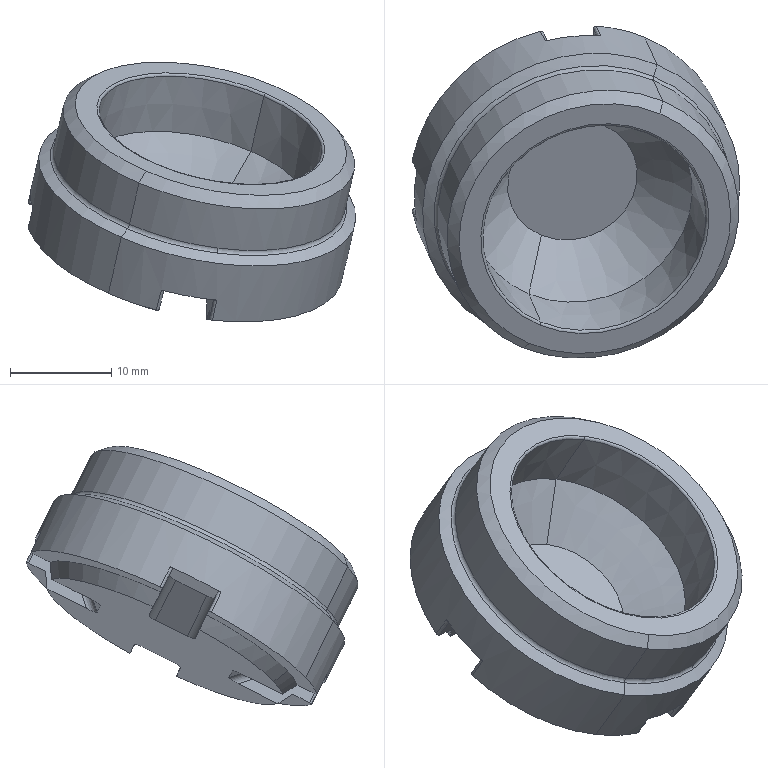Part | SolidWorks | features BaseBody 1 | 1 solid | 62 faces | box 32.369 x 32.817 x 25.668 mm | volume 6352 mm3 | plane 23 | cone 14 | cylinder 12 | spline 8 | torus 5 | commonest cylinder face diameters 1.6 x8 29.4 x2 32 x2